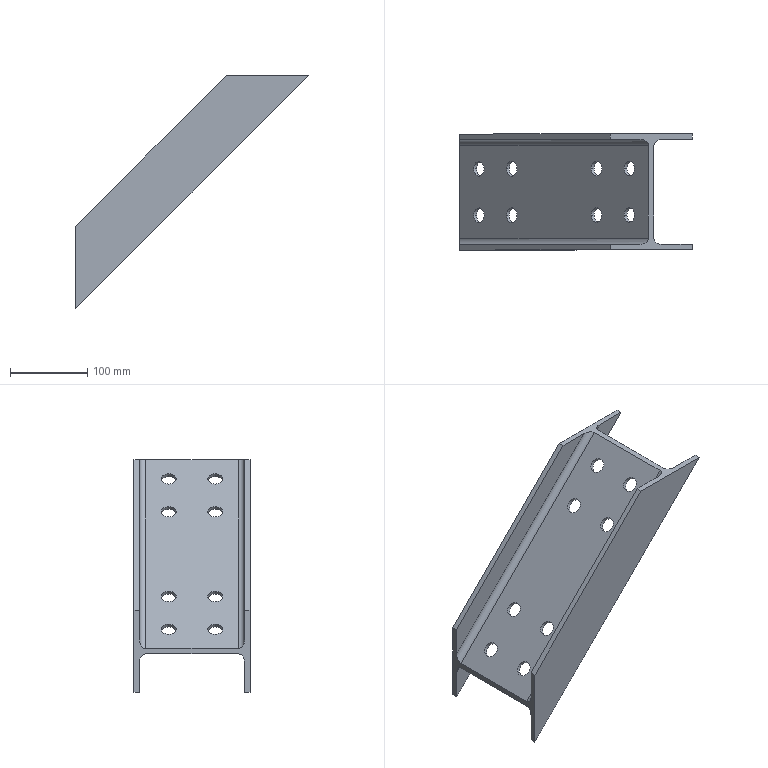Part | STEP file | 计量Diagonal Brace梁1_Default<As Machined> | 1 solid | 34 faces | box 300.52 x 150 x 300.52 mm | volume 613387 mm3 | cylinder 20 | plane 14 | commonest cylinder face diameters 19 x16 16 x4